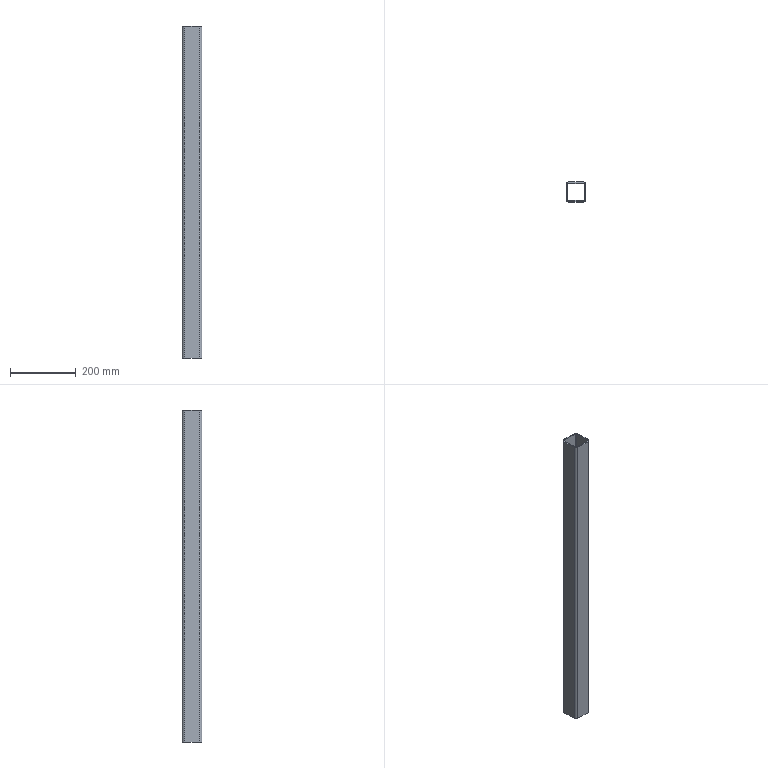Part | SolidWorks | features ICE 1, LibraryFeature 1 | 1 solid | 18 faces | box 60 x 60 x 1010 mm | volume 863344 mm3 | plane 10 | cylinder 8 | commonest cylinder face diameters 8 x4 16 x4
STEP:
#1=CARTESIAN_POINT('',(22.,30.,0.));
#2=VERTEX_POINT('',#1);
#3=CARTESIAN_POINT('',(-22.,30.,0.));
#4=VERTEX_POINT('',#3);
#5=CARTESIAN_POINT('',(0.,30.,0.));
#6=DIRECTION('',(-1.,0.,0.));
#7=VECTOR('',#6,1000.);
#8=LINE('',#5,#7);
#9=EDGE_CURVE('',#2,#4,#8,.T.);
#10=ORIENTED_EDGE('',*,*,#9,.T.);
#11=CARTESIAN_POINT('',(-22.,30.,1010.));
#12=VERTEX_POINT('',#11);
#13=CARTESIAN_POINT('',(-22.,30.,1010.));
#14=DIRECTION('',(0.,0.,-1.));
#15=VECTOR('',#14,1000.);
#16=LINE('',#13,#15);
#17=EDGE_CURVE('',#12,#4,#16,.T.);
#18=ORIENTED_EDGE('',*,*,#17,.F.);
#19=CARTESIAN_POINT('',(22.,30.,1010.));
#20=VERTEX_POINT('',#19);
#21=CARTESIAN_POINT('',(0.,30.,1010.));
#22=DIRECTION('',(-1.,0.,0.));
#23=VECTOR('',#22,1000.);
#24=LINE('',#21,#23);
#25=EDGE_CURVE('',#20,#12,#24,.T.);
#26=ORIENTED_EDGE('',*,*,#25,.F.);
#27=CARTESIAN_POINT('',(22.,30.,1010.));
#28=DIRECTION('',(0.,0.,-1.));
#29=VECTOR('',#28,1000.);
#30=LINE('',#27,#29);
#31=EDGE_CURVE('',#20,#2,#30,.T.);
#32=ORIENTED_EDGE('',*,*,#31,.T.);
#33=EDGE_LOOP('',(#10,#18,#26,#32));
#34=FACE_OUTER_BOUND('',#33,.T.);
#35=CARTESIAN_POINT('',(0.,30.,1010.));
#36=DIRECTION('',(0.,-1.,0.));
#37=DIRECTION('',(0.,0.,-1.));
#38=AXIS2_PLACEMENT_3D('',#35,#36,#37);
#39=PLANE('',#38);
#40=ADVANCED_FACE('',(#34),#39,.F.);
#41=CARTESIAN_POINT('',(-30.,22.,0.));
#42=VERTEX_POINT('',#41);
#43=CARTESIAN_POINT('',(-22.,22.,0.));
#44=DIRECTION('',(0.,0.,1.));
#45=DIRECTION('',(1.,0.,0.));
#46=AXIS2_PLACEMENT_3D('',#43,#44,#45);
#47=CIRCLE('',#46,8.);
#48=EDGE_CURVE('',#4,#42,#47,.T.);
#49=ORIENTED_EDGE('',*,*,#48,.T.);
#50=CARTESIAN_POINT('',(-30.,22.,1010.));
#51=VERTEX_POINT('',#50);
#52=CARTESIAN_POINT('',(-30.,22.,1010.));
#53=DIRECTION('',(0.,0.,-1.));
#54=VECTOR('',#53,1000.);
#55=LINE('',#52,#54);
#56=EDGE_CURVE('',#51,#42,#55,.T.);
#57=ORIENTED_EDGE('',*,*,#56,.F.);
#58=CARTESIAN_POINT('',(-22.,22.,1010.));
#59=DIRECTION('',(0.,0.,1.));
#60=DIRECTION('',(1.,0.,0.));
#61=AXIS2_PLACEMENT_3D('',#58,#59,#60);
#62=CIRCLE('',#61,8.);
#63=EDGE_CURVE('',#12,#51,#62,.T.);
#64=ORIENTED_EDGE('',*,*,#63,.F.);
#65=ORIENTED_EDGE('',*,*,#17,.T.);
#66=EDGE_LOOP('',(#49,#57,#64,#65));
#67=FACE_OUTER_BOUND('',#66,.T.);
#68=CARTESIAN_POINT('',(-22.,22.,1010.));
#69=DIRECTION('',(0.,0.,-1.));
#70=DIRECTION('',(-1.,0.,0.));
#71=AXIS2_PLACEMENT_3D('',#68,#69,#70);
#72=CYLINDRICAL_SURFACE('',#71,8.);
#73=ADVANCED_FACE('',(#67),#72,.T.);
#74=CARTESIAN_POINT('',(-30.,-22.,0.));
#75=VERTEX_POINT('',#74);
#76=CARTESIAN_POINT('',(-30.,0.,0.));
#77=DIRECTION('',(0.,1.,0.));
#78=VECTOR('',#77,1000.);
#79=LINE('',#76,#78);
#80=EDGE_CURVE('',#75,#42,#79,.T.);
#81=ORIENTED_EDGE('',*,*,#80,.F.);
#82=CARTESIAN_POINT('',(-30.,-22.,1010.));
#83=VERTEX_POINT('',#82);
#84=CARTESIAN_POINT('',(-30.,-22.,1010.));
#85=DIRECTION('',(0.,0.,-1.));
#86=VECTOR('',#85,1000.);
#87=LINE('',#84,#86);
#88=EDGE_CURVE('',#83,#75,#87,.T.);
#89=ORIENTED_EDGE('',*,*,#88,.F.);
#90=CARTESIAN_POINT('',(-30.,0.,1010.));
#91=DIRECTION('',(0.,1.,0.));
#92=VECTOR('',#91,1000.);
#93=LINE('',#90,#92);
#94=EDGE_CURVE('',#83,#51,#93,.T.);
#95=ORIENTED_EDGE('',*,*,#94,.T.);
#96=ORIENTED_EDGE('',*,*,#56,.T.);
#97=EDGE_LOOP('',(#81,#89,#95,#96));
#98=FACE_OUTER_BOUND('',#97,.T.);
#99=CARTESIAN_POINT('',(-30.,0.,1010.));
#100=DIRECTION('',(-1.,0.,0.));
#101=DIRECTION('',(0.,0.,1.));
#102=AXIS2_PLACEMENT_3D('',#99,#100,#101);
#103=PLANE('',#102);
#104=ADVANCED_FACE('',(#98),#103,.T.);
#105=CARTESIAN_POINT('',(-22.,-30.,0.));
#106=VERTEX_POINT('',#105);
#107=CARTESIAN_POINT('',(-22.,-22.,0.));
#108=DIRECTION('',(0.,0.,1.));
#109=DIRECTION('',(1.,0.,0.));
#110=AXIS2_PLACEMENT_3D('',#107,#108,#109);
#111=CIRCLE('',#110,8.);
#112=EDGE_CURVE('',#75,#106,#111,.T.);
#113=ORIENTED_EDGE('',*,*,#112,.T.);
#114=CARTESIAN_POINT('',(-22.,-30.,1010.));
#115=VERTEX_POINT('',#114);
#116=CARTESIAN_POINT('',(-22.,-30.,1010.));
#117=DIRECTION('',(0.,0.,-1.));
#118=VECTOR('',#117,1000.);
#119=LINE('',#116,#118);
#120=EDGE_CURVE('',#115,#106,#119,.T.);
#121=ORIENTED_EDGE('',*,*,#120,.F.);
#122=CARTESIAN_POINT('',(-22.,-22.,1010.));
#123=DIRECTION('',(0.,0.,1.));
#124=DIRECTION('',(1.,0.,0.));
#125=AXIS2_PLACEMENT_3D('',#122,#123,#124);
#126=CIRCLE('',#125,8.);
#127=EDGE_CURVE('',#83,#115,#126,.T.);
#128=ORIENTED_EDGE('',*,*,#127,.F.);
#129=ORIENTED_EDGE('',*,*,#88,.T.);
#130=EDGE_LOOP('',(#113,#121,#128,#129));
#131=FACE_OUTER_BOUND('',#130,.T.);
#132=CARTESIAN_POINT('',(-22.,-22.,1010.));
#133=DIRECTION('',(0.,0.,-1.));
#134=DIRECTION('',(-1.,0.,0.));
#135=AXIS2_PLACEMENT_3D('',#132,#133,#134);
#136=CYLINDRICAL_SURFACE('',#135,8.);
#137=ADVANCED_FACE('',(#131),#136,.T.);
#138=CARTESIAN_POINT('',(22.,-30.,0.));
#139=VERTEX_POINT('',#138);
#140=CARTESIAN_POINT('',(0.,-30.,0.));
#141=DIRECTION('',(1.,0.,0.));
#142=VECTOR('',#141,1000.);
#143=LINE('',#140,#142);
#144=EDGE_CURVE('',#106,#139,#143,.T.);
#145=ORIENTED_EDGE('',*,*,#144,.T.);
#146=CARTESIAN_POINT('',(22.,-30.,1010.));
#147=VERTEX_POINT('',#146);
#148=CARTESIAN_POINT('',(22.,-30.,1010.));
#149=DIRECTION('',(0.,0.,-1.));
#150=VECTOR('',#149,1000.);
#151=LINE('',#148,#150);
#152=EDGE_CURVE('',#147,#139,#151,.T.);
#153=ORIENTED_EDGE('',*,*,#152,.F.);
#154=CARTESIAN_POINT('',(0.,-30.,1010.));
#155=DIRECTION('',(1.,0.,0.));
#156=VECTOR('',#155,1000.);
#157=LINE('',#154,#156);
#158=EDGE_CURVE('',#115,#147,#157,.T.);
#159=ORIENTED_EDGE('',*,*,#158,.F.);
#160=ORIENTED_EDGE('',*,*,#120,.T.);
#161=EDGE_LOOP('',(#145,#153,#159,#160));
#162=FACE_OUTER_BOUND('',#161,.T.);
#163=CARTESIAN_POINT('',(0.,-30.,1010.));
#164=DIRECTION('',(0.,1.,0.));
#165=DIRECTION('',(0.,0.,1.));
#166=AXIS2_PLACEMENT_3D('',#163,#164,#165);
#167=PLANE('',#166);
#168=ADVANCED_FACE('',(#162),#167,.F.);
#169=CARTESIAN_POINT('',(30.,-22.,0.));
#170=VERTEX_POINT('',#169);
#171=CARTESIAN_POINT('',(22.,-22.,0.));
#172=DIRECTION('',(0.,0.,1.));
#173=DIRECTION('',(1.,0.,0.));
#174=AXIS2_PLACEMENT_3D('',#171,#172,#173);
#175=CIRCLE('',#174,8.);
#176=EDGE_CURVE('',#139,#170,#175,.T.);
#177=ORIENTED_EDGE('',*,*,#176,.T.);
#178=CARTESIAN_POINT('',(30.,-22.,1010.));
#179=VERTEX_POINT('',#178);
#180=CARTESIAN_POINT('',(30.,-22.,1010.));
#181=DIRECTION('',(0.,0.,-1.));
#182=VECTOR('',#181,1000.);
#183=LINE('',#180,#182);
#184=EDGE_CURVE('',#179,#170,#183,.T.);
#185=ORIENTED_EDGE('',*,*,#184,.F.);
#186=CARTESIAN_POINT('',(22.,-22.,1010.));
#187=DIRECTION('',(0.,0.,1.));
#188=DIRECTION('',(1.,0.,0.));
#189=AXIS2_PLACEMENT_3D('',#186,#187,#188);
#190=CIRCLE('',#189,8.);
#191=EDGE_CURVE('',#147,#179,#190,.T.);
#192=ORIENTED_EDGE('',*,*,#191,.F.);
#193=ORIENTED_EDGE('',*,*,#152,.T.);
#194=EDGE_LOOP('',(#177,#185,#192,#193));
#195=FACE_OUTER_BOUND('',#194,.T.);
#196=CARTESIAN_POINT('',(22.,-22.,1010.));
#197=DIRECTION('',(0.,0.,-1.));
#198=DIRECTION('',(-1.,0.,0.));
#199=AXIS2_PLACEMENT_3D('',#196,#197,#198);
#200=CYLINDRICAL_SURFACE('',#199,8.);
#201=ADVANCED_FACE('',(#195),#200,.T.);
#202=CARTESIAN_POINT('',(30.,22.,0.));
#203=VERTEX_POINT('',#202);
#204=CARTESIAN_POINT('',(30.,0.,0.));
#205=DIRECTION('',(0.,-1.,0.));
#206=VECTOR('',#205,1000.);
#207=LINE('',#204,#206);
#208=EDGE_CURVE('',#203,#170,#207,.T.);
#209=ORIENTED_EDGE('',*,*,#208,.F.);
#210=CARTESIAN_POINT('',(30.,22.,1010.));
#211=VERTEX_POINT('',#210);
#212=CARTESIAN_POINT('',(30.,22.,1010.));
#213=DIRECTION('',(0.,0.,-1.));
#214=VECTOR('',#213,1000.);
#215=LINE('',#212,#214);
#216=EDGE_CURVE('',#211,#203,#215,.T.);
#217=ORIENTED_EDGE('',*,*,#216,.F.);
#218=CARTESIAN_POINT('',(30.,0.,1010.));
#219=DIRECTION('',(0.,-1.,0.));
#220=VECTOR('',#219,1000.);
#221=LINE('',#218,#220);
#222=EDGE_CURVE('',#211,#179,#221,.T.);
#223=ORIENTED_EDGE('',*,*,#222,.T.);
#224=ORIENTED_EDGE('',*,*,#184,.T.);
#225=EDGE_LOOP('',(#209,#217,#223,#224));
#226=FACE_OUTER_BOUND('',#225,.T.);
#227=CARTESIAN_POINT('',(30.,0.,1010.));
#228=DIRECTION('',(1.,0.,0.));
#229=DIRECTION('',(0.,0.,-1.));
#230=AXIS2_PLACEMENT_3D('',#227,#228,#229);
#231=PLANE('',#230);
#232=ADVANCED_FACE('',(#226),#231,.T.);
#233=CARTESIAN_POINT('',(-26.,-22.,0.));
#234=VERTEX_POINT('',#233);
#235=CARTESIAN_POINT('',(-22.,-26.,0.));
#236=VERTEX_POINT('',#235);
#237=CARTESIAN_POINT('',(-22.,-22.,0.));
#238=DIRECTION('',(0.,0.,1.));
#239=DIRECTION('',(1.,0.,0.));
#240=AXIS2_PLACEMENT_3D('',#237,#238,#239);
#241=CIRCLE('',#240,4.);
#242=EDGE_CURVE('',#234,#236,#241,.T.);
#243=ORIENTED_EDGE('',*,*,#242,.F.);
#244=CARTESIAN_POINT('',(-26.,-22.,1010.));
#245=VERTEX_POINT('',#244);
#246=CARTESIAN_POINT('',(-26.,-22.,1010.));
#247=DIRECTION('',(0.,0.,-1.));
#248=VECTOR('',#247,1000.);
#249=LINE('',#246,#248);
#250=EDGE_CURVE('',#245,#234,#249,.T.);
#251=ORIENTED_EDGE('',*,*,#250,.F.);
#252=CARTESIAN_POINT('',(-22.,-26.,1010.));
#253=VERTEX_POINT('',#252);
#254=CARTESIAN_POINT('',(-22.,-22.,1010.));
#255=DIRECTION('',(0.,0.,1.));
#256=DIRECTION('',(1.,0.,0.));
#257=AXIS2_PLACEMENT_3D('',#254,#255,#256);
#258=CIRCLE('',#257,4.);
#259=EDGE_CURVE('',#245,#253,#258,.T.);
#260=ORIENTED_EDGE('',*,*,#259,.T.);
#261=CARTESIAN_POINT('',(-22.,-26.,1010.));
#262=DIRECTION('',(0.,0.,-1.));
#263=VECTOR('',#262,1000.);
#264=LINE('',#261,#263);
#265=EDGE_CURVE('',#253,#236,#264,.T.);
#266=ORIENTED_EDGE('',*,*,#265,.T.);
#267=EDGE_LOOP('',(#243,#251,#260,#266));
#268=FACE_OUTER_BOUND('',#267,.T.);
#269=CARTESIAN_POINT('',(-22.,-22.,1010.));
#270=DIRECTION('',(0.,0.,-1.));
#271=DIRECTION('',(-1.,0.,0.));
#272=AXIS2_PLACEMENT_3D('',#269,#270,#271);
#273=CYLINDRICAL_SURFACE('',#272,4.);
#274=ADVANCED_FACE('',(#268),#273,.F.);
#275=CARTESIAN_POINT('',(-26.,22.,0.));
#276=VERTEX_POINT('',#275);
#277=CARTESIAN_POINT('',(-26.,0.,0.));
#278=DIRECTION('',(0.,1.,0.));
#279=VECTOR('',#278,1000.);
#280=LINE('',#277,#279);
#281=EDGE_CURVE('',#234,#276,#280,.T.);
#282=ORIENTED_EDGE('',*,*,#281,.T.);
#283=CARTESIAN_POINT('',(-26.,22.,1010.));
#284=VERTEX_POINT('',#283);
#285=CARTESIAN_POINT('',(-26.,22.,1010.));
#286=DIRECTION('',(0.,0.,-1.));
#287=VECTOR('',#286,1000.);
#288=LINE('',#285,#287);
#289=EDGE_CURVE('',#284,#276,#288,.T.);
#290=ORIENTED_EDGE('',*,*,#289,.F.);
#291=CARTESIAN_POINT('',(-26.,0.,1010.));
#292=DIRECTION('',(0.,1.,0.));
#293=VECTOR('',#292,1000.);
#294=LINE('',#291,#293);
#295=EDGE_CURVE('',#245,#284,#294,.T.);
#296=ORIENTED_EDGE('',*,*,#295,.F.);
#297=ORIENTED_EDGE('',*,*,#250,.T.);
#298=EDGE_LOOP('',(#282,#290,#296,#297));
#299=FACE_OUTER_BOUND('',#298,.T.);
#300=CARTESIAN_POINT('',(-26.,0.,1010.));
#301=DIRECTION('',(-1.,0.,0.));
#302=DIRECTION('',(0.,0.,1.));
#303=AXIS2_PLACEMENT_3D('',#300,#301,#302);
#304=PLANE('',#303);
#305=ADVANCED_FACE('',(#299),#304,.F.);
#306=CARTESIAN_POINT('',(-22.,26.,0.));
#307=VERTEX_POINT('',#306);
#308=CARTESIAN_POINT('',(-22.,22.,0.));
#309=DIRECTION('',(0.,0.,1.));
#310=DIRECTION('',(1.,0.,0.));
#311=AXIS2_PLACEMENT_3D('',#308,#309,#310);
#312=CIRCLE('',#311,4.);
#313=EDGE_CURVE('',#307,#276,#312,.T.);
#314=ORIENTED_EDGE('',*,*,#313,.F.);
#315=CARTESIAN_POINT('',(-22.,26.,1010.));
#316=VERTEX_POINT('',#315);
#317=CARTESIAN_POINT('',(-22.,26.,1010.));
#318=DIRECTION('',(0.,0.,-1.));
#319=VECTOR('',#318,1000.);
#320=LINE('',#317,#319);
#321=EDGE_CURVE('',#316,#307,#320,.T.);
#322=ORIENTED_EDGE('',*,*,#321,.F.);
#323=CARTESIAN_POINT('',(-22.,22.,1010.));
#324=DIRECTION('',(0.,0.,1.));
#325=DIRECTION('',(1.,0.,0.));
#326=AXIS2_PLACEMENT_3D('',#323,#324,#325);
#327=CIRCLE('',#326,4.);
#328=EDGE_CURVE('',#316,#284,#327,.T.);
#329=ORIENTED_EDGE('',*,*,#328,.T.);
#330=ORIENTED_EDGE('',*,*,#289,.T.);
#331=EDGE_LOOP('',(#314,#322,#329,#330));
#332=FACE_OUTER_BOUND('',#331,.T.);
#333=CARTESIAN_POINT('',(-22.,22.,1010.));
#334=DIRECTION('',(0.,0.,-1.));
#335=DIRECTION('',(-1.,0.,0.));
#336=AXIS2_PLACEMENT_3D('',#333,#334,#335);
#337=CYLINDRICAL_SURFACE('',#336,4.);
#338=ADVANCED_FACE('',(#332),#337,.F.);
#339=CARTESIAN_POINT('',(22.,26.,0.));
#340=VERTEX_POINT('',#339);
#341=CARTESIAN_POINT('',(0.,26.,0.));
#342=DIRECTION('',(-1.,0.,0.));
#343=VECTOR('',#342,1000.);
#344=LINE('',#341,#343);
#345=EDGE_CURVE('',#340,#307,#344,.T.);
#346=ORIENTED_EDGE('',*,*,#345,.F.);
#347=CARTESIAN_POINT('',(22.,26.,1010.));
#348=VERTEX_POINT('',#347);
#349=CARTESIAN_POINT('',(22.,26.,1010.));
#350=DIRECTION('',(0.,0.,-1.));
#351=VECTOR('',#350,1000.);
#352=LINE('',#349,#351);
#353=EDGE_CURVE('',#348,#340,#352,.T.);
#354=ORIENTED_EDGE('',*,*,#353,.F.);
#355=CARTESIAN_POINT('',(0.,26.,1010.));
#356=DIRECTION('',(-1.,0.,0.));
#357=VECTOR('',#356,1000.);
#358=LINE('',#355,#357);
#359=EDGE_CURVE('',#348,#316,#358,.T.);
#360=ORIENTED_EDGE('',*,*,#359,.T.);
#361=ORIENTED_EDGE('',*,*,#321,.T.);
#362=EDGE_LOOP('',(#346,#354,#360,#361));
#363=FACE_OUTER_BOUND('',#362,.T.);
#364=CARTESIAN_POINT('',(0.,26.,1010.));
#365=DIRECTION('',(0.,-1.,0.));
#366=DIRECTION('',(0.,0.,-1.));
#367=AXIS2_PLACEMENT_3D('',#364,#365,#366);
#368=PLANE('',#367);
#369=ADVANCED_FACE('',(#363),#368,.T.);
#370=CARTESIAN_POINT('',(26.,22.,0.));
#371=VERTEX_POINT('',#370);
#372=CARTESIAN_POINT('',(22.,22.,0.));
#373=DIRECTION('',(0.,0.,1.));
#374=DIRECTION('',(1.,0.,0.));
#375=AXIS2_PLACEMENT_3D('',#372,#373,#374);
#376=CIRCLE('',#375,4.);
#377=EDGE_CURVE('',#371,#340,#376,.T.);
#378=ORIENTED_EDGE('',*,*,#377,.F.);
#379=CARTESIAN_POINT('',(26.,22.,1010.));
#380=VERTEX_POINT('',#379);
#381=CARTESIAN_POINT('',(26.,22.,1010.));
#382=DIRECTION('',(0.,0.,-1.));
#383=VECTOR('',#382,1000.);
#384=LINE('',#381,#383);
#385=EDGE_CURVE('',#380,#371,#384,.T.);
#386=ORIENTED_EDGE('',*,*,#385,.F.);
#387=CARTESIAN_POINT('',(22.,22.,1010.));
#388=DIRECTION('',(0.,0.,1.));
#389=DIRECTION('',(1.,0.,0.));
#390=AXIS2_PLACEMENT_3D('',#387,#388,#389);
#391=CIRCLE('',#390,4.);
#392=EDGE_CURVE('',#380,#348,#391,.T.);
#393=ORIENTED_EDGE('',*,*,#392,.T.);
#394=ORIENTED_EDGE('',*,*,#353,.T.);
#395=EDGE_LOOP('',(#378,#386,#393,#394));
#396=FACE_OUTER_BOUND('',#395,.T.);
#397=CARTESIAN_POINT('',(22.,22.,1010.));
#398=DIRECTION('',(0.,0.,-1.));
#399=DIRECTION('',(-1.,0.,0.));
#400=AXIS2_PLACEMENT_3D('',#397,#398,#399);
#401=CYLINDRICAL_SURFACE('',#400,4.);
#402=ADVANCED_FACE('',(#396),#401,.F.);
#403=CARTESIAN_POINT('',(26.,-22.,0.));
#404=VERTEX_POINT('',#403);
#405=CARTESIAN_POINT('',(26.,0.,0.));
#406=DIRECTION('',(0.,-1.,0.));
#407=VECTOR('',#406,1000.);
#408=LINE('',#405,#407);
#409=EDGE_CURVE('',#371,#404,#408,.T.);
#410=ORIENTED_EDGE('',*,*,#409,.T.);
#411=CARTESIAN_POINT('',(26.,-22.,1010.));
#412=VERTEX_POINT('',#411);
#413=CARTESIAN_POINT('',(26.,-22.,1010.));
#414=DIRECTION('',(0.,0.,-1.));
#415=VECTOR('',#414,1000.);
#416=LINE('',#413,#415);
#417=EDGE_CURVE('',#412,#404,#416,.T.);
#418=ORIENTED_EDGE('',*,*,#417,.F.);
#419=CARTESIAN_POINT('',(26.,0.,1010.));
#420=DIRECTION('',(0.,-1.,0.));
#421=VECTOR('',#420,1000.);
#422=LINE('',#419,#421);
#423=EDGE_CURVE('',#380,#412,#422,.T.);
#424=ORIENTED_EDGE('',*,*,#423,.F.);
#425=ORIENTED_EDGE('',*,*,#385,.T.);
#426=EDGE_LOOP('',(#410,#418,#424,#425));
#427=FACE_OUTER_BOUND('',#426,.T.);
#428=CARTESIAN_POINT('',(26.,0.,1010.));
#429=DIRECTION('',(1.,0.,0.));
#430=DIRECTION('',(0.,0.,-1.));
#431=AXIS2_PLACEMENT_3D('',#428,#429,#430);
#432=PLANE('',#431);
#433=ADVANCED_FACE('',(#427),#432,.F.);
#434=CARTESIAN_POINT('',(22.,-26.,0.));
#435=VERTEX_POINT('',#434);
#436=CARTESIAN_POINT('',(22.,-22.,0.));
#437=DIRECTION('',(0.,0.,1.));
#438=DIRECTION('',(1.,0.,0.));
#439=AXIS2_PLACEMENT_3D('',#436,#437,#438);
#440=CIRCLE('',#439,4.);
#441=EDGE_CURVE('',#435,#404,#440,.T.);
#442=ORIENTED_EDGE('',*,*,#441,.F.);
#443=CARTESIAN_POINT('',(22.,-26.,1010.));
#444=VERTEX_POINT('',#443);
#445=CARTESIAN_POINT('',(22.,-26.,1010.));
#446=DIRECTION('',(0.,0.,-1.));
#447=VECTOR('',#446,1000.);
#448=LINE('',#445,#447);
#449=EDGE_CURVE('',#444,#435,#448,.T.);
#450=ORIENTED_EDGE('',*,*,#449,.F.);
#451=CARTESIAN_POINT('',(22.,-22.,1010.));
#452=DIRECTION('',(0.,0.,1.));
#453=DIRECTION('',(1.,0.,0.));
#454=AXIS2_PLACEMENT_3D('',#451,#452,#453);
#455=CIRCLE('',#454,4.);
#456=EDGE_CURVE('',#444,#412,#455,.T.);
#457=ORIENTED_EDGE('',*,*,#456,.T.);
#458=ORIENTED_EDGE('',*,*,#417,.T.);
#459=EDGE_LOOP('',(#442,#450,#457,#458));
#460=FACE_OUTER_BOUND('',#459,.T.);
#461=CARTESIAN_POINT('',(22.,-22.,1010.));
#462=DIRECTION('',(0.,0.,-1.));
#463=DIRECTION('',(-1.,0.,0.));
#464=AXIS2_PLACEMENT_3D('',#461,#462,#463);
#465=CYLINDRICAL_SURFACE('',#464,4.);
#466=ADVANCED_FACE('',(#460),#465,.F.);
#467=CARTESIAN_POINT('',(0.,-26.,0.));
#468=DIRECTION('',(1.,0.,0.));
#469=VECTOR('',#468,1000.);
#470=LINE('',#467,#469);
#471=EDGE_CURVE('',#236,#435,#470,.T.);
#472=ORIENTED_EDGE('',*,*,#471,.F.);
#473=ORIENTED_EDGE('',*,*,#265,.F.);
#474=CARTESIAN_POINT('',(0.,-26.,1010.));
#475=DIRECTION('',(1.,0.,0.));
#476=VECTOR('',#475,1000.);
#477=LINE('',#474,#476);
#478=EDGE_CURVE('',#253,#444,#477,.T.);
#479=ORIENTED_EDGE('',*,*,#478,.T.);
#480=ORIENTED_EDGE('',*,*,#449,.T.);
#481=EDGE_LOOP('',(#472,#473,#479,#480));
#482=FACE_OUTER_BOUND('',#481,.T.);
#483=CARTESIAN_POINT('',(0.,-26.,1010.));
#484=DIRECTION('',(0.,1.,0.));
#485=DIRECTION('',(0.,0.,1.));
#486=AXIS2_PLACEMENT_3D('',#483,#484,#485);
#487=PLANE('',#486);
#488=ADVANCED_FACE('',(#482),#487,.T.);
#489=CARTESIAN_POINT('',(22.,22.,0.));
#490=DIRECTION('',(0.,0.,1.));
#491=DIRECTION('',(1.,0.,0.));
#492=AXIS2_PLACEMENT_3D('',#489,#490,#491);
#493=CIRCLE('',#492,8.);
#494=EDGE_CURVE('',#203,#2,#493,.T.);
#495=ORIENTED_EDGE('',*,*,#494,.T.);
#496=ORIENTED_EDGE('',*,*,#31,.F.);
#497=CARTESIAN_POINT('',(22.,22.,1010.));
#498=DIRECTION('',(0.,0.,1.));
#499=DIRECTION('',(1.,0.,0.));
#500=AXIS2_PLACEMENT_3D('',#497,#498,#499);
#501=CIRCLE('',#500,8.);
#502=EDGE_CURVE('',#211,#20,#501,.T.);
#503=ORIENTED_EDGE('',*,*,#502,.F.);
#504=ORIENTED_EDGE('',*,*,#216,.T.);
#505=EDGE_LOOP('',(#495,#496,#503,#504));
#506=FACE_OUTER_BOUND('',#505,.T.);
#507=CARTESIAN_POINT('',(22.,22.,1010.));
#508=DIRECTION('',(0.,0.,-1.));
#509=DIRECTION('',(-1.,0.,0.));
#510=AXIS2_PLACEMENT_3D('',#507,#508,#509);
#511=CYLINDRICAL_SURFACE('',#510,8.);
#512=ADVANCED_FACE('',(#506),#511,.T.);
#513=ORIENTED_EDGE('',*,*,#259,.F.);
#514=ORIENTED_EDGE('',*,*,#295,.T.);
#515=ORIENTED_EDGE('',*,*,#328,.F.);
#516=ORIENTED_EDGE('',*,*,#359,.F.);
#517=ORIENTED_EDGE('',*,*,#392,.F.);
#518=ORIENTED_EDGE('',*,*,#423,.T.);
#519=ORIENTED_EDGE('',*,*,#456,.F.);
#520=ORIENTED_EDGE('',*,*,#478,.F.);
#521=EDGE_LOOP('',(#513,#514,#515,#516,#517,#518,#519,#520));
#522=FACE_BOUND('',#521,.T.);
#523=ORIENTED_EDGE('',*,*,#25,.T.);
#524=ORIENTED_EDGE('',*,*,#63,.T.);
#525=ORIENTED_EDGE('',*,*,#94,.F.);
#526=ORIENTED_EDGE('',*,*,#127,.T.);
#527=ORIENTED_EDGE('',*,*,#158,.T.);
#528=ORIENTED_EDGE('',*,*,#191,.T.);
#529=ORIENTED_EDGE('',*,*,#222,.F.);
#530=ORIENTED_EDGE('',*,*,#502,.T.);
#531=EDGE_LOOP('',(#523,#524,#525,#526,#527,#528,#529,#530));
#532=FACE_OUTER_BOUND('',#531,.T.);
#533=CARTESIAN_POINT('',(0.,0.,1010.));
#534=DIRECTION('',(0.,0.,1.));
#535=DIRECTION('',(1.,0.,0.));
#536=AXIS2_PLACEMENT_3D('',#533,#534,#535);
#537=PLANE('',#536);
#538=ADVANCED_FACE('',(#522,#532),#537,.T.);
#539=ORIENTED_EDGE('',*,*,#242,.T.);
#540=ORIENTED_EDGE('',*,*,#471,.T.);
#541=ORIENTED_EDGE('',*,*,#441,.T.);
#542=ORIENTED_EDGE('',*,*,#409,.F.);
#543=ORIENTED_EDGE('',*,*,#377,.T.);
#544=ORIENTED_EDGE('',*,*,#345,.T.);
#545=ORIENTED_EDGE('',*,*,#313,.T.);
#546=ORIENTED_EDGE('',*,*,#281,.F.);
#547=EDGE_LOOP('',(#539,#540,#541,#542,#543,#544,#545,#546));
#548=FACE_BOUND('',#547,.T.);
#549=ORIENTED_EDGE('',*,*,#9,.F.);
#550=ORIENTED_EDGE('',*,*,#494,.F.);
#551=ORIENTED_EDGE('',*,*,#208,.T.);
#552=ORIENTED_EDGE('',*,*,#176,.F.);
#553=ORIENTED_EDGE('',*,*,#144,.F.);
#554=ORIENTED_EDGE('',*,*,#112,.F.);
#555=ORIENTED_EDGE('',*,*,#80,.T.);
#556=ORIENTED_EDGE('',*,*,#48,.F.);
#557=EDGE_LOOP('',(#549,#550,#551,#552,#553,#554,#555,#556));
#558=FACE_OUTER_BOUND('',#557,.T.);
#559=CARTESIAN_POINT('',(0.,0.,0.));
#560=DIRECTION('',(0.,0.,1.));
#561=DIRECTION('',(1.,0.,0.));
#562=AXIS2_PLACEMENT_3D('',#559,#560,#561);
#563=PLANE('',#562);
#564=ADVANCED_FACE('',(#548,#558),#563,.F.);
#565=CLOSED_SHELL('',(#40,#73,#104,#137,#168,#201,#232,#274,#305,#338,#369,#402,#433,#466,#488,#512,#538,#564));
#566=MANIFOLD_SOLID_BREP('',#565);
#567=CARTESIAN_POINT('',(0.,0.,0.));
#568=DIRECTION('',(0.,0.,1.));
#569=DIRECTION('',(1.,0.,0.));
#570=AXIS2_PLACEMENT_3D('',#567,#568,#569);
#571=(LENGTH_UNIT()NAMED_UNIT(*)SI_UNIT(.MILLI.,.METRE.));
#572=UNCERTAINTY_MEASURE_WITH_UNIT(LENGTH_MEASURE(0.00001),#571,'','');
#573=(NAMED_UNIT(*)PLANE_ANGLE_UNIT()SI_UNIT($,.RADIAN.));
#574=(NAMED_UNIT(*)SI_UNIT($,.STERADIAN.)SOLID_ANGLE_UNIT());
#575=(GEOMETRIC_REPRESENTATION_CONTEXT(3)GLOBAL_UNCERTAINTY_ASSIGNED_CONTEXT((#572))GLOBAL_UNIT_ASSIGNED_CONTEXT((#571,#573,#574))REPRESENTATION_CONTEXT('',''));
#576=ADVANCED_BREP_SHAPE_REPRESENTATION('',(#566,#570),#575);